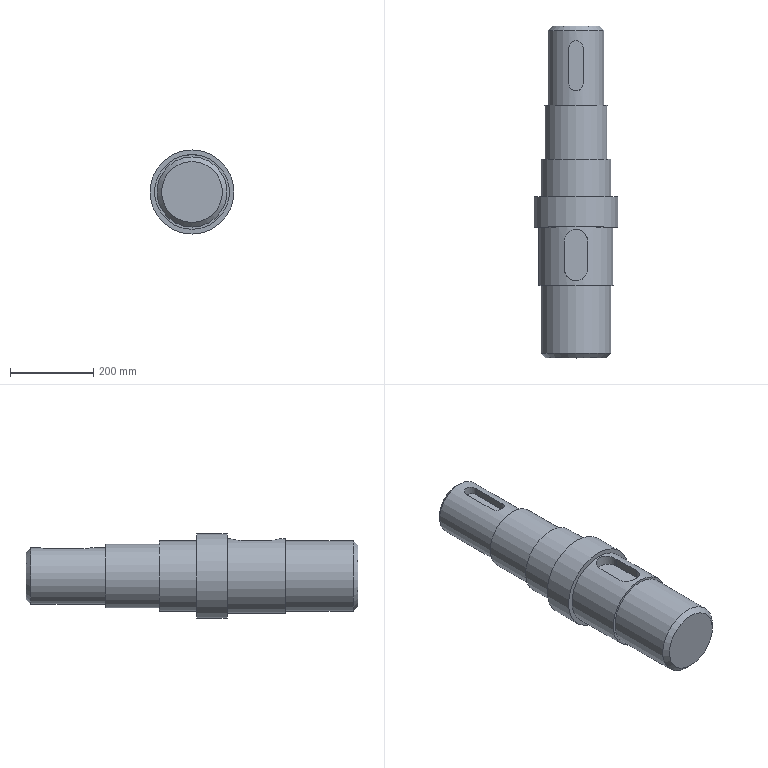Part | NX | features BOSS 5, CHAMFER 2, DATUM_PLANE 2, RECT_SLOT 2, CYLINDER 1, DATUM_CSYS 1, Delete Body 1, LINKED_BODY 1, MOVE_FACE 1, SCALE 1 | 1 solid | 25 faces | box 202.5 x 798.75 x 202.5 mm | volume 16646925 mm3 | plane 13 | cylinder 10 | cone 2 | commonest cylinder face diameters 33.75 x2 56.25 x2 168.75 x2 135 x1 151.875 x1 180 x1
STEP:
#1=CARTESIAN_POINT('',(-1724.979,434.125,-310.332));
#2=VERTEX_POINT('',#1);
#3=CARTESIAN_POINT('',(-1724.979,434.125,-366.582));
#4=DIRECTION('',(0.,1.,0.));
#5=DIRECTION('',(0.,0.,1.));
#6=AXIS2_PLACEMENT_3D('',#3,#4,#5);
#7=CIRCLE('',#6,56.25);
#8=EDGE_CURVE('',#2,#2,#7,.T.);
#9=ORIENTED_EDGE('',*,*,#8,.T.);
#10=EDGE_LOOP('',(#9));
#11=FACE_BOUND('',#10,.T.);
#12=CARTESIAN_POINT('',(-1724.979,434.125,-366.582));
#13=DIRECTION('',(0.,1.,0.));
#14=DIRECTION('',(0.,0.,1.));
#15=AXIS2_PLACEMENT_3D('',#12,#13,#14);
#16=PLANE('',#15);
#17=ADVANCED_FACE('',(#11),#16,.T.);
#18=CARTESIAN_POINT('',(-1741.854,381.851,-301.226));
#19=VERTEX_POINT('',#18);
#20=CARTESIAN_POINT('',(-1741.854,294.976,-301.226));
#21=VERTEX_POINT('',#20);
#22=CARTESIAN_POINT('',(-1741.854,242.875,-301.226));
#23=DIRECTION('',(0.,1.,0.));
#24=VECTOR('',#23,1000.);
#25=LINE('',#22,#24);
#26=EDGE_CURVE('',#19,#21,#25,.F.);
#27=ORIENTED_EDGE('',*,*,#26,.F.);
#28=CARTESIAN_POINT('',(-1708.104,381.851,-301.226));
#29=VERTEX_POINT('',#28);
#30=CARTESIAN_POINT('',(-1708.104,381.851,-301.226));
#31=CARTESIAN_POINT('',(-1708.104,384.09,-301.226));
#32=CARTESIAN_POINT('',(-1708.995,388.496,-300.987));
#33=CARTESIAN_POINT('',(-1712.741,394.093,-300.143));
#34=CARTESIAN_POINT('',(-1718.323,397.833,-299.314));
#35=CARTESIAN_POINT('',(-1724.963,399.17,-298.968));
#36=CARTESIAN_POINT('',(-1731.612,397.845,-299.309));
#37=CARTESIAN_POINT('',(-1739.094,392.847,-300.43));
#38=CARTESIAN_POINT('',(-1741.854,386.329,-301.226));
#39=CARTESIAN_POINT('',(-1741.854,381.851,-301.226));
#40=B_SPLINE_CURVE_WITH_KNOTS('',3,(#30,#31,#32,#33,#34,#35,#36,#37,#38,#39),.UNSPECIFIED.,.F.,.F.,(4,1,1,1,1,1,1,4),(0.,0.006619,0.01324,0.01986,0.02648,0.0331,0.03971,0.05295),.UNSPECIFIED.);
#41=EDGE_CURVE('',#29,#19,#40,.T.);
#42=ORIENTED_EDGE('',*,*,#41,.F.);
#43=CARTESIAN_POINT('',(-1708.104,294.976,-301.226));
#44=VERTEX_POINT('',#43);
#45=CARTESIAN_POINT('',(-1708.104,242.875,-301.226));
#46=DIRECTION('',(0.,1.,0.));
#47=VECTOR('',#46,1000.);
#48=LINE('',#45,#47);
#49=EDGE_CURVE('',#44,#29,#48,.T.);
#50=ORIENTED_EDGE('',*,*,#49,.F.);
#51=CARTESIAN_POINT('',(-1741.854,294.976,-301.226));
#52=CARTESIAN_POINT('',(-1741.854,292.737,-301.226));
#53=CARTESIAN_POINT('',(-1740.964,288.332,-300.987));
#54=CARTESIAN_POINT('',(-1737.218,282.735,-300.143));
#55=CARTESIAN_POINT('',(-1731.636,278.995,-299.314));
#56=CARTESIAN_POINT('',(-1724.996,277.658,-298.968));
#57=CARTESIAN_POINT('',(-1718.347,278.983,-299.309));
#58=CARTESIAN_POINT('',(-1710.865,283.981,-300.43));
#59=CARTESIAN_POINT('',(-1708.104,290.498,-301.226));
#60=CARTESIAN_POINT('',(-1708.104,294.976,-301.226));
#61=B_SPLINE_CURVE_WITH_KNOTS('',3,(#51,#52,#53,#54,#55,#56,#57,#58,#59,#60),.UNSPECIFIED.,.F.,.F.,(4,1,1,1,1,1,1,4),(0.,0.006619,0.01324,0.01986,0.02648,0.0331,0.03971,0.05295),.UNSPECIFIED.);
#62=EDGE_CURVE('',#21,#44,#61,.T.);
#63=ORIENTED_EDGE('',*,*,#62,.F.);
#64=EDGE_LOOP('',(#27,#42,#50,#63));
#65=FACE_BOUND('',#64,.T.);
#66=CARTESIAN_POINT('',(-1724.979,422.875,-299.082));
#67=VERTEX_POINT('',#66);
#68=CARTESIAN_POINT('',(-1724.979,422.875,-366.582));
#69=DIRECTION('',(0.,1.,0.));
#70=DIRECTION('',(0.,0.,1.));
#71=AXIS2_PLACEMENT_3D('',#68,#69,#70);
#72=CIRCLE('',#71,67.5);
#73=EDGE_CURVE('',#67,#67,#72,.F.);
#74=ORIENTED_EDGE('',*,*,#73,.T.);
#75=EDGE_LOOP('',(#74));
#76=FACE_BOUND('',#75,.T.);
#77=CARTESIAN_POINT('',(-1724.979,242.875,-299.082));
#78=VERTEX_POINT('',#77);
#79=CARTESIAN_POINT('',(-1724.979,242.875,-366.582));
#80=DIRECTION('',(0.,1.,0.));
#81=DIRECTION('',(0.,0.,1.));
#82=AXIS2_PLACEMENT_3D('',#79,#80,#81);
#83=CIRCLE('',#82,67.5);
#84=EDGE_CURVE('',#78,#78,#83,.F.);
#85=ORIENTED_EDGE('',*,*,#84,.F.);
#86=EDGE_LOOP('',(#85));
#87=FACE_BOUND('',#86,.T.);
#88=CARTESIAN_POINT('',(-1724.979,242.875,-366.582));
#89=DIRECTION('',(0.,1.,0.));
#90=DIRECTION('',(0.,0.,1.));
#91=AXIS2_PLACEMENT_3D('',#88,#89,#90);
#92=CYLINDRICAL_SURFACE('',#91,67.5);
#93=ADVANCED_FACE('',(#65,#76,#87),#92,.T.);
#94=ORIENTED_EDGE('',*,*,#84,.T.);
#95=EDGE_LOOP('',(#94));
#96=FACE_BOUND('',#95,.T.);
#97=CARTESIAN_POINT('',(-1724.979,242.875,-442.52));
#98=VERTEX_POINT('',#97);
#99=CARTESIAN_POINT('',(-1724.979,242.875,-366.582));
#100=DIRECTION('',(0.,-1.,0.));
#101=DIRECTION('',(0.,0.,-1.));
#102=AXIS2_PLACEMENT_3D('',#99,#100,#101);
#103=CIRCLE('',#102,75.938);
#104=EDGE_CURVE('',#98,#98,#103,.T.);
#105=ORIENTED_EDGE('',*,*,#104,.F.);
#106=EDGE_LOOP('',(#105));
#107=FACE_BOUND('',#106,.T.);
#108=CARTESIAN_POINT('',(-1724.979,242.875,-366.582));
#109=DIRECTION('',(0.,1.,0.));
#110=DIRECTION('',(0.,0.,1.));
#111=AXIS2_PLACEMENT_3D('',#108,#109,#110);
#112=PLANE('',#111);
#113=ADVANCED_FACE('',(#96,#107),#112,.T.);
#114=CARTESIAN_POINT('',(-1724.979,113.5,-442.52));
#115=VERTEX_POINT('',#114);
#116=CARTESIAN_POINT('',(-1724.979,113.5,-366.582));
#117=DIRECTION('',(0.,-1.,0.));
#118=DIRECTION('',(0.,0.,-1.));
#119=AXIS2_PLACEMENT_3D('',#116,#117,#118);
#120=CIRCLE('',#119,75.938);
#121=EDGE_CURVE('',#115,#115,#120,.T.);
#122=ORIENTED_EDGE('',*,*,#121,.F.);
#123=EDGE_LOOP('',(#122));
#124=FACE_BOUND('',#123,.T.);
#125=ORIENTED_EDGE('',*,*,#104,.T.);
#126=EDGE_LOOP('',(#125));
#127=FACE_BOUND('',#126,.T.);
#128=CARTESIAN_POINT('',(-1724.979,242.875,-366.582));
#129=DIRECTION('',(0.,-1.,0.));
#130=DIRECTION('',(0.,0.,-1.));
#131=AXIS2_PLACEMENT_3D('',#128,#129,#130);
#132=CYLINDRICAL_SURFACE('',#131,75.938);
#133=ADVANCED_FACE('',(#124,#127),#132,.T.);
#134=ORIENTED_EDGE('',*,*,#121,.T.);
#135=EDGE_LOOP('',(#134));
#136=FACE_BOUND('',#135,.T.);
#137=CARTESIAN_POINT('',(-1724.979,113.5,-450.957));
#138=VERTEX_POINT('',#137);
#139=CARTESIAN_POINT('',(-1724.979,113.5,-366.582));
#140=DIRECTION('',(0.,-1.,0.));
#141=DIRECTION('',(0.,0.,-1.));
#142=AXIS2_PLACEMENT_3D('',#139,#140,#141);
#143=CIRCLE('',#142,84.375);
#144=EDGE_CURVE('',#138,#138,#143,.T.);
#145=ORIENTED_EDGE('',*,*,#144,.F.);
#146=EDGE_LOOP('',(#145));
#147=FACE_BOUND('',#146,.T.);
#148=CARTESIAN_POINT('',(-1724.979,113.5,-366.582));
#149=DIRECTION('',(0.,1.,0.));
#150=DIRECTION('',(0.,0.,1.));
#151=AXIS2_PLACEMENT_3D('',#148,#149,#150);
#152=PLANE('',#151);
#153=ADVANCED_FACE('',(#136,#147),#152,.T.);
#154=CARTESIAN_POINT('',(-1724.979,23.5,-450.957));
#155=VERTEX_POINT('',#154);
#156=CARTESIAN_POINT('',(-1724.979,23.5,-366.582));
#157=DIRECTION('',(0.,-1.,0.));
#158=DIRECTION('',(0.,0.,-1.));
#159=AXIS2_PLACEMENT_3D('',#156,#157,#158);
#160=CIRCLE('',#159,84.375);
#161=EDGE_CURVE('',#155,#155,#160,.T.);
#162=ORIENTED_EDGE('',*,*,#161,.F.);
#163=EDGE_LOOP('',(#162));
#164=FACE_BOUND('',#163,.T.);
#165=ORIENTED_EDGE('',*,*,#144,.T.);
#166=EDGE_LOOP('',(#165));
#167=FACE_BOUND('',#166,.T.);
#168=CARTESIAN_POINT('',(-1724.979,113.5,-366.582));
#169=DIRECTION('',(0.,-1.,0.));
#170=DIRECTION('',(0.,0.,-1.));
#171=AXIS2_PLACEMENT_3D('',#168,#169,#170);
#172=CYLINDRICAL_SURFACE('',#171,84.375);
#173=ADVANCED_FACE('',(#164,#167),#172,.T.);
#174=CARTESIAN_POINT('',(-1724.979,-49.625,-456.582));
#175=VERTEX_POINT('',#174);
#176=CARTESIAN_POINT('',(-1724.979,-49.625,-366.582));
#177=DIRECTION('',(0.,-1.,0.));
#178=DIRECTION('',(0.,0.,-1.));
#179=AXIS2_PLACEMENT_3D('',#176,#177,#178);
#180=CIRCLE('',#179,90.);
#181=EDGE_CURVE('',#175,#175,#180,.T.);
#182=ORIENTED_EDGE('',*,*,#181,.F.);
#183=EDGE_LOOP('',(#182));
#184=FACE_BOUND('',#183,.T.);
#185=CARTESIAN_POINT('',(-1724.979,-49.625,-467.832));
#186=VERTEX_POINT('',#185);
#187=CARTESIAN_POINT('',(-1724.979,-49.625,-366.582));
#188=DIRECTION('',(0.,-1.,0.));
#189=DIRECTION('',(0.,0.,-1.));
#190=AXIS2_PLACEMENT_3D('',#187,#188,#189);
#191=CIRCLE('',#190,101.25);
#192=EDGE_CURVE('',#186,#186,#191,.T.);
#193=ORIENTED_EDGE('',*,*,#192,.T.);
#194=EDGE_LOOP('',(#193));
#195=FACE_BOUND('',#194,.T.);
#196=CARTESIAN_POINT('',(-1724.979,-49.625,-366.582));
#197=DIRECTION('',(0.,-1.,0.));
#198=DIRECTION('',(0.,0.,-1.));
#199=AXIS2_PLACEMENT_3D('',#196,#197,#198);
#200=PLANE('',#199);
#201=ADVANCED_FACE('',(#184,#195),#200,.T.);
#202=ORIENTED_EDGE('',*,*,#161,.T.);
#203=EDGE_LOOP('',(#202));
#204=FACE_BOUND('',#203,.T.);
#205=CARTESIAN_POINT('',(-1724.979,23.5,-467.832));
#206=VERTEX_POINT('',#205);
#207=CARTESIAN_POINT('',(-1724.979,23.5,-366.582));
#208=DIRECTION('',(0.,-1.,0.));
#209=DIRECTION('',(0.,0.,-1.));
#210=AXIS2_PLACEMENT_3D('',#207,#208,#209);
#211=CIRCLE('',#210,101.25);
#212=EDGE_CURVE('',#206,#206,#211,.T.);
#213=ORIENTED_EDGE('',*,*,#212,.F.);
#214=EDGE_LOOP('',(#213));
#215=FACE_BOUND('',#214,.T.);
#216=CARTESIAN_POINT('',(-1724.979,23.5,-366.582));
#217=DIRECTION('',(0.,1.,0.));
#218=DIRECTION('',(0.,0.,1.));
#219=AXIS2_PLACEMENT_3D('',#216,#217,#218);
#220=PLANE('',#219);
#221=ADVANCED_FACE('',(#204,#215),#220,.T.);
#222=ORIENTED_EDGE('',*,*,#192,.F.);
#223=EDGE_LOOP('',(#222));
#224=FACE_BOUND('',#223,.T.);
#225=ORIENTED_EDGE('',*,*,#212,.T.);
#226=EDGE_LOOP('',(#225));
#227=FACE_BOUND('',#226,.T.);
#228=CARTESIAN_POINT('',(-1724.979,23.5,-366.582));
#229=DIRECTION('',(0.,-1.,0.));
#230=DIRECTION('',(0.,0.,-1.));
#231=AXIS2_PLACEMENT_3D('',#228,#229,#230);
#232=CYLINDRICAL_SURFACE('',#231,101.25);
#233=ADVANCED_FACE('',(#224,#227),#232,.T.);
#234=CARTESIAN_POINT('',(-1724.979,-190.25,-450.957));
#235=VERTEX_POINT('',#234);
#236=CARTESIAN_POINT('',(-1724.979,-190.25,-366.582));
#237=DIRECTION('',(0.,-1.,0.));
#238=DIRECTION('',(0.,0.,-1.));
#239=AXIS2_PLACEMENT_3D('',#236,#237,#238);
#240=CIRCLE('',#239,84.375);
#241=EDGE_CURVE('',#235,#235,#240,.T.);
#242=ORIENTED_EDGE('',*,*,#241,.F.);
#243=EDGE_LOOP('',(#242));
#244=FACE_BOUND('',#243,.T.);
#245=CARTESIAN_POINT('',(-1724.979,-190.25,-456.582));
#246=VERTEX_POINT('',#245);
#247=CARTESIAN_POINT('',(-1724.979,-190.25,-366.582));
#248=DIRECTION('',(0.,-1.,0.));
#249=DIRECTION('',(0.,0.,-1.));
#250=AXIS2_PLACEMENT_3D('',#247,#248,#249);
#251=CIRCLE('',#250,90.);
#252=EDGE_CURVE('',#246,#246,#251,.T.);
#253=ORIENTED_EDGE('',*,*,#252,.T.);
#254=EDGE_LOOP('',(#253));
#255=FACE_BOUND('',#254,.T.);
#256=CARTESIAN_POINT('',(-1724.979,-190.25,-366.582));
#257=DIRECTION('',(0.,-1.,0.));
#258=DIRECTION('',(0.,0.,-1.));
#259=AXIS2_PLACEMENT_3D('',#256,#257,#258);
#260=PLANE('',#259);
#261=ADVANCED_FACE('',(#244,#255),#260,.T.);
#262=CARTESIAN_POINT('',(-1753.104,-83.375,-281.09));
#263=VERTEX_POINT('',#262);
#264=CARTESIAN_POINT('',(-1753.104,-150.875,-281.09));
#265=VERTEX_POINT('',#264);
#266=CARTESIAN_POINT('',(-1753.104,-49.625,-281.09));
#267=DIRECTION('',(0.,-1.,0.));
#268=VECTOR('',#267,1000.);
#269=LINE('',#266,#268);
#270=EDGE_CURVE('',#263,#265,#269,.T.);
#271=ORIENTED_EDGE('',*,*,#270,.F.);
#272=CARTESIAN_POINT('',(-1696.854,-83.375,-281.09));
#273=VERTEX_POINT('',#272);
#274=CARTESIAN_POINT('',(-1696.854,-83.375,-281.09));
#275=CARTESIAN_POINT('',(-1696.854,-81.505,-281.09));
#276=CARTESIAN_POINT('',(-1697.219,-77.839,-280.968));
#277=CARTESIAN_POINT('',(-1699.392,-70.704,-280.278));
#278=CARTESIAN_POINT('',(-1704.582,-62.985,-278.802));
#279=CARTESIAN_POINT('',(-1713.861,-56.747,-277.066));
#280=CARTESIAN_POINT('',(-1724.946,-54.506,-276.342));
#281=CARTESIAN_POINT('',(-1736.061,-56.727,-277.06));
#282=CARTESIAN_POINT('',(-1745.375,-62.976,-278.8));
#283=CARTESIAN_POINT('',(-1751.603,-72.261,-280.575));
#284=CARTESIAN_POINT('',(-1753.104,-79.634,-281.09));
#285=CARTESIAN_POINT('',(-1753.104,-83.375,-281.09));
#286=B_SPLINE_CURVE_WITH_KNOTS('',3,(#274,#275,#276,#277,#278,#279,#280,#281,#282,#283,#284,#285),.UNSPECIFIED.,.F.,.F.,(4,1,1,1,1,1,1,1,1,4),(0.,0.005528,0.01106,0.02211,0.03317,0.04423,0.05528,0.06634,0.0774,0.08846),.UNSPECIFIED.);
#287=EDGE_CURVE('',#273,#263,#286,.T.);
#288=ORIENTED_EDGE('',*,*,#287,.F.);
#289=CARTESIAN_POINT('',(-1696.854,-150.875,-281.09));
#290=VERTEX_POINT('',#289);
#291=CARTESIAN_POINT('',(-1696.854,-49.625,-281.09));
#292=DIRECTION('',(0.,-1.,0.));
#293=VECTOR('',#292,1000.);
#294=LINE('',#291,#293);
#295=EDGE_CURVE('',#290,#273,#294,.F.);
#296=ORIENTED_EDGE('',*,*,#295,.F.);
#297=CARTESIAN_POINT('',(-1753.104,-150.875,-281.09));
#298=CARTESIAN_POINT('',(-1753.104,-152.745,-281.09));
#299=CARTESIAN_POINT('',(-1752.739,-156.411,-280.968));
#300=CARTESIAN_POINT('',(-1750.567,-163.546,-280.278));
#301=CARTESIAN_POINT('',(-1745.377,-171.265,-278.802));
#302=CARTESIAN_POINT('',(-1736.097,-177.503,-277.066));
#303=CARTESIAN_POINT('',(-1725.013,-179.744,-276.342));
#304=CARTESIAN_POINT('',(-1713.897,-177.523,-277.06));
#305=CARTESIAN_POINT('',(-1704.583,-171.274,-278.8));
#306=CARTESIAN_POINT('',(-1698.356,-161.989,-280.575));
#307=CARTESIAN_POINT('',(-1696.854,-154.616,-281.09));
#308=CARTESIAN_POINT('',(-1696.854,-150.875,-281.09));
#309=B_SPLINE_CURVE_WITH_KNOTS('',3,(#297,#298,#299,#300,#301,#302,#303,#304,#305,#306,#307,#308),.UNSPECIFIED.,.F.,.F.,(4,1,1,1,1,1,1,1,1,4),(0.,0.005528,0.01106,0.02211,0.03317,0.04423,0.05528,0.06634,0.0774,0.08846),.UNSPECIFIED.);
#310=EDGE_CURVE('',#265,#290,#309,.T.);
#311=ORIENTED_EDGE('',*,*,#310,.F.);
#312=EDGE_LOOP('',(#271,#288,#296,#311));
#313=FACE_BOUND('',#312,.T.);
#314=ORIENTED_EDGE('',*,*,#252,.F.);
#315=EDGE_LOOP('',(#314));
#316=FACE_BOUND('',#315,.T.);
#317=ORIENTED_EDGE('',*,*,#181,.T.);
#318=EDGE_LOOP('',(#317));
#319=FACE_BOUND('',#318,.T.);
#320=CARTESIAN_POINT('',(-1724.979,-49.625,-366.582));
#321=DIRECTION('',(0.,-1.,0.));
#322=DIRECTION('',(0.,0.,-1.));
#323=AXIS2_PLACEMENT_3D('',#320,#321,#322);
#324=CYLINDRICAL_SURFACE('',#323,90.);
#325=ADVANCED_FACE('',(#313,#316,#319),#324,.T.);
#326=CARTESIAN_POINT('',(-1724.979,-364.625,-439.707));
#327=VERTEX_POINT('',#326);
#328=CARTESIAN_POINT('',(-1724.979,-364.625,-366.582));
#329=DIRECTION('',(0.,-1.,0.));
#330=DIRECTION('',(0.,0.,-1.));
#331=AXIS2_PLACEMENT_3D('',#328,#329,#330);
#332=CIRCLE('',#331,73.125);
#333=EDGE_CURVE('',#327,#327,#332,.T.);
#334=ORIENTED_EDGE('',*,*,#333,.T.);
#335=EDGE_LOOP('',(#334));
#336=FACE_BOUND('',#335,.T.);
#337=CARTESIAN_POINT('',(-1724.979,-364.625,-366.582));
#338=DIRECTION('',(0.,-1.,0.));
#339=DIRECTION('',(0.,0.,-1.));
#340=AXIS2_PLACEMENT_3D('',#337,#338,#339);
#341=PLANE('',#340);
#342=ADVANCED_FACE('',(#336),#341,.T.);
#343=CARTESIAN_POINT('',(-1724.979,-353.375,-450.957));
#344=VERTEX_POINT('',#343);
#345=CARTESIAN_POINT('',(-1724.979,-353.375,-366.582));
#346=DIRECTION('',(0.,-1.,0.));
#347=DIRECTION('',(0.,0.,-1.));
#348=AXIS2_PLACEMENT_3D('',#345,#346,#347);
#349=CIRCLE('',#348,84.375);
#350=EDGE_CURVE('',#344,#344,#349,.F.);
#351=ORIENTED_EDGE('',*,*,#350,.T.);
#352=EDGE_LOOP('',(#351));
#353=FACE_BOUND('',#352,.T.);
#354=ORIENTED_EDGE('',*,*,#241,.T.);
#355=EDGE_LOOP('',(#354));
#356=FACE_BOUND('',#355,.T.);
#357=CARTESIAN_POINT('',(-1724.979,-190.25,-366.582));
#358=DIRECTION('',(0.,-1.,0.));
#359=DIRECTION('',(0.,0.,-1.));
#360=AXIS2_PLACEMENT_3D('',#357,#358,#359);
#361=CYLINDRICAL_SURFACE('',#360,84.375);
#362=ADVANCED_FACE('',(#353,#356),#361,.T.);
#363=ORIENTED_EDGE('',*,*,#350,.F.);
#364=EDGE_LOOP('',(#363));
#365=FACE_BOUND('',#364,.T.);
#366=ORIENTED_EDGE('',*,*,#333,.F.);
#367=EDGE_LOOP('',(#366));
#368=FACE_BOUND('',#367,.T.);
#369=CARTESIAN_POINT('',(-1724.979,-364.625,-366.582));
#370=DIRECTION('',(0.,1.,0.));
#371=DIRECTION('',(0.,0.,1.));
#372=AXIS2_PLACEMENT_3D('',#369,#370,#371);
#373=CONICAL_SURFACE('',#372,73.125,0.7854);
#374=ADVANCED_FACE('',(#365,#368),#373,.T.);
#375=ORIENTED_EDGE('',*,*,#8,.F.);
#376=EDGE_LOOP('',(#375));
#377=FACE_BOUND('',#376,.T.);
#378=ORIENTED_EDGE('',*,*,#73,.F.);
#379=EDGE_LOOP('',(#378));
#380=FACE_BOUND('',#379,.T.);
#381=CARTESIAN_POINT('',(-1724.979,422.875,-366.582));
#382=DIRECTION('',(0.,-1.,0.));
#383=DIRECTION('',(0.,0.,-1.));
#384=AXIS2_PLACEMENT_3D('',#381,#382,#383);
#385=CONICAL_SURFACE('',#384,67.5,0.7854);
#386=ADVANCED_FACE('',(#377,#380),#385,.T.);
#387=ORIENTED_EDGE('',*,*,#26,.T.);
#388=CARTESIAN_POINT('',(-1741.854,294.976,-318.77));
#389=VERTEX_POINT('',#388);
#390=CARTESIAN_POINT('',(-1741.854,294.976,-299.082));
#391=DIRECTION('',(0.,0.,1.));
#392=VECTOR('',#391,1000.);
#393=LINE('',#390,#392);
#394=EDGE_CURVE('',#21,#389,#393,.F.);
#395=ORIENTED_EDGE('',*,*,#394,.T.);
#396=CARTESIAN_POINT('',(-1741.854,381.851,-318.77));
#397=VERTEX_POINT('',#396);
#398=CARTESIAN_POINT('',(-1741.854,274.976,-318.77));
#399=DIRECTION('',(0.,1.,0.));
#400=VECTOR('',#399,1000.);
#401=LINE('',#398,#400);
#402=EDGE_CURVE('',#397,#389,#401,.F.);
#403=ORIENTED_EDGE('',*,*,#402,.F.);
#404=CARTESIAN_POINT('',(-1741.854,381.851,-299.082));
#405=DIRECTION('',(0.,0.,1.));
#406=VECTOR('',#405,1000.);
#407=LINE('',#404,#406);
#408=EDGE_CURVE('',#19,#397,#407,.F.);
#409=ORIENTED_EDGE('',*,*,#408,.F.);
#410=EDGE_LOOP('',(#387,#395,#403,#409));
#411=FACE_BOUND('',#410,.T.);
#412=CARTESIAN_POINT('',(-1741.854,328.414,-299.082));
#413=DIRECTION('',(-1.,0.,0.));
#414=DIRECTION('',(0.,0.,1.));
#415=AXIS2_PLACEMENT_3D('',#412,#413,#414);
#416=PLANE('',#415);
#417=ADVANCED_FACE('',(#411),#416,.F.);
#418=ORIENTED_EDGE('',*,*,#402,.T.);
#419=CARTESIAN_POINT('',(-1708.104,294.976,-318.77));
#420=VERTEX_POINT('',#419);
#421=CARTESIAN_POINT('',(-1724.979,294.976,-318.77));
#422=DIRECTION('',(0.,0.,1.));
#423=DIRECTION('',(1.,0.,0.));
#424=AXIS2_PLACEMENT_3D('',#421,#422,#423);
#425=CIRCLE('',#424,16.875);
#426=EDGE_CURVE('',#420,#389,#425,.F.);
#427=ORIENTED_EDGE('',*,*,#426,.F.);
#428=CARTESIAN_POINT('',(-1708.104,381.851,-318.77));
#429=VERTEX_POINT('',#428);
#430=CARTESIAN_POINT('',(-1708.104,274.976,-318.77));
#431=DIRECTION('',(0.,1.,0.));
#432=VECTOR('',#431,1000.);
#433=LINE('',#430,#432);
#434=EDGE_CURVE('',#429,#420,#433,.F.);
#435=ORIENTED_EDGE('',*,*,#434,.F.);
#436=CARTESIAN_POINT('',(-1724.979,381.851,-318.77));
#437=DIRECTION('',(0.,0.,1.));
#438=DIRECTION('',(1.,0.,0.));
#439=AXIS2_PLACEMENT_3D('',#436,#437,#438);
#440=CIRCLE('',#439,16.875);
#441=EDGE_CURVE('',#397,#429,#440,.F.);
#442=ORIENTED_EDGE('',*,*,#441,.F.);
#443=EDGE_LOOP('',(#418,#427,#435,#442));
#444=FACE_BOUND('',#443,.T.);
#445=CARTESIAN_POINT('',(-1724.979,328.414,-318.77));
#446=DIRECTION('',(0.,0.,-1.));
#447=DIRECTION('',(-1.,0.,0.));
#448=AXIS2_PLACEMENT_3D('',#445,#446,#447);
#449=PLANE('',#448);
#450=ADVANCED_FACE('',(#444),#449,.F.);
#451=ORIENTED_EDGE('',*,*,#394,.F.);
#452=ORIENTED_EDGE('',*,*,#62,.T.);
#453=CARTESIAN_POINT('',(-1708.104,294.976,-299.082));
#454=DIRECTION('',(0.,0.,1.));
#455=VECTOR('',#454,1000.);
#456=LINE('',#453,#455);
#457=EDGE_CURVE('',#44,#420,#456,.F.);
#458=ORIENTED_EDGE('',*,*,#457,.T.);
#459=ORIENTED_EDGE('',*,*,#426,.T.);
#460=EDGE_LOOP('',(#451,#452,#458,#459));
#461=FACE_BOUND('',#460,.T.);
#462=CARTESIAN_POINT('',(-1724.979,294.976,-299.082));
#463=DIRECTION('',(0.,0.,1.));
#464=DIRECTION('',(1.,0.,0.));
#465=AXIS2_PLACEMENT_3D('',#462,#463,#464);
#466=CYLINDRICAL_SURFACE('',#465,16.875);
#467=ADVANCED_FACE('',(#461),#466,.F.);
#468=ORIENTED_EDGE('',*,*,#49,.T.);
#469=CARTESIAN_POINT('',(-1708.104,381.851,-299.082));
#470=DIRECTION('',(0.,0.,1.));
#471=VECTOR('',#470,1000.);
#472=LINE('',#469,#471);
#473=EDGE_CURVE('',#29,#429,#472,.F.);
#474=ORIENTED_EDGE('',*,*,#473,.T.);
#475=ORIENTED_EDGE('',*,*,#434,.T.);
#476=ORIENTED_EDGE('',*,*,#457,.F.);
#477=EDGE_LOOP('',(#468,#474,#475,#476));
#478=FACE_BOUND('',#477,.T.);
#479=CARTESIAN_POINT('',(-1708.104,328.414,-299.082));
#480=DIRECTION('',(1.,0.,0.));
#481=DIRECTION('',(0.,0.,-1.));
#482=AXIS2_PLACEMENT_3D('',#479,#480,#481);
#483=PLANE('',#482);
#484=ADVANCED_FACE('',(#478),#483,.F.);
#485=ORIENTED_EDGE('',*,*,#473,.F.);
#486=ORIENTED_EDGE('',*,*,#41,.T.);
#487=ORIENTED_EDGE('',*,*,#408,.T.);
#488=ORIENTED_EDGE('',*,*,#441,.T.);
#489=EDGE_LOOP('',(#485,#486,#487,#488));
#490=FACE_BOUND('',#489,.T.);
#491=CARTESIAN_POINT('',(-1724.979,381.851,-299.082));
#492=DIRECTION('',(0.,0.,1.));
#493=DIRECTION('',(1.,0.,0.));
#494=AXIS2_PLACEMENT_3D('',#491,#492,#493);
#495=CYLINDRICAL_SURFACE('',#494,16.875);
#496=ADVANCED_FACE('',(#490),#495,.F.);
#497=ORIENTED_EDGE('',*,*,#270,.T.);
#498=CARTESIAN_POINT('',(-1753.104,-150.875,-301.895));
#499=VERTEX_POINT('',#498);
#500=CARTESIAN_POINT('',(-1753.104,-150.875,-276.582));
#501=DIRECTION('',(0.,0.,1.));
#502=VECTOR('',#501,1000.);
#503=LINE('',#500,#502);
#504=EDGE_CURVE('',#265,#499,#503,.F.);
#505=ORIENTED_EDGE('',*,*,#504,.T.);
#506=CARTESIAN_POINT('',(-1753.104,-83.375,-301.895));
#507=VERTEX_POINT('',#506);
#508=CARTESIAN_POINT('',(-1753.104,-150.875,-301.895));
#509=DIRECTION('',(0.,1.,0.));
#510=VECTOR('',#509,1000.);
#511=LINE('',#508,#510);
#512=EDGE_CURVE('',#507,#499,#511,.F.);
#513=ORIENTED_EDGE('',*,*,#512,.F.);
#514=CARTESIAN_POINT('',(-1753.104,-83.375,-276.582));
#515=DIRECTION('',(0.,0.,1.));
#516=VECTOR('',#515,1000.);
#517=LINE('',#514,#516);
#518=EDGE_CURVE('',#263,#507,#517,.F.);
#519=ORIENTED_EDGE('',*,*,#518,.F.);
#520=EDGE_LOOP('',(#497,#505,#513,#519));
#521=FACE_BOUND('',#520,.T.);
#522=CARTESIAN_POINT('',(-1753.104,-117.125,-276.582));
#523=DIRECTION('',(-1.,0.,0.));
#524=DIRECTION('',(0.,0.,1.));
#525=AXIS2_PLACEMENT_3D('',#522,#523,#524);
#526=PLANE('',#525);
#527=ADVANCED_FACE('',(#521),#526,.F.);
#528=ORIENTED_EDGE('',*,*,#512,.T.);
#529=CARTESIAN_POINT('',(-1696.854,-150.875,-301.895));
#530=VERTEX_POINT('',#529);
#531=CARTESIAN_POINT('',(-1724.979,-150.875,-301.895));
#532=DIRECTION('',(0.,0.,1.));
#533=DIRECTION('',(1.,0.,0.));
#534=AXIS2_PLACEMENT_3D('',#531,#532,#533);
#535=CIRCLE('',#534,28.125);
#536=EDGE_CURVE('',#530,#499,#535,.F.);
#537=ORIENTED_EDGE('',*,*,#536,.F.);
#538=CARTESIAN_POINT('',(-1696.854,-83.375,-301.895));
#539=VERTEX_POINT('',#538);
#540=CARTESIAN_POINT('',(-1696.854,-150.875,-301.895));
#541=DIRECTION('',(0.,1.,0.));
#542=VECTOR('',#541,1000.);
#543=LINE('',#540,#542);
#544=EDGE_CURVE('',#539,#530,#543,.F.);
#545=ORIENTED_EDGE('',*,*,#544,.F.);
#546=CARTESIAN_POINT('',(-1724.979,-83.375,-301.895));
#547=DIRECTION('',(0.,0.,1.));
#548=DIRECTION('',(1.,0.,0.));
#549=AXIS2_PLACEMENT_3D('',#546,#547,#548);
#550=CIRCLE('',#549,28.125);
#551=EDGE_CURVE('',#507,#539,#550,.F.);
#552=ORIENTED_EDGE('',*,*,#551,.F.);
#553=EDGE_LOOP('',(#528,#537,#545,#552));
#554=FACE_BOUND('',#553,.T.);
#555=CARTESIAN_POINT('',(-1724.979,-117.125,-301.895));
#556=DIRECTION('',(0.,0.,-1.));
#557=DIRECTION('',(-1.,0.,0.));
#558=AXIS2_PLACEMENT_3D('',#555,#556,#557);
#559=PLANE('',#558);
#560=ADVANCED_FACE('',(#554),#559,.F.);
#561=ORIENTED_EDGE('',*,*,#504,.F.);
#562=ORIENTED_EDGE('',*,*,#310,.T.);
#563=CARTESIAN_POINT('',(-1696.854,-150.875,-276.582));
#564=DIRECTION('',(0.,0.,1.));
#565=VECTOR('',#564,1000.);
#566=LINE('',#563,#565);
#567=EDGE_CURVE('',#290,#530,#566,.F.);
#568=ORIENTED_EDGE('',*,*,#567,.T.);
#569=ORIENTED_EDGE('',*,*,#536,.T.);
#570=EDGE_LOOP('',(#561,#562,#568,#569));
#571=FACE_BOUND('',#570,.T.);
#572=CARTESIAN_POINT('',(-1724.979,-150.875,-276.582));
#573=DIRECTION('',(0.,0.,1.));
#574=DIRECTION('',(1.,0.,0.));
#575=AXIS2_PLACEMENT_3D('',#572,#573,#574);
#576=CYLINDRICAL_SURFACE('',#575,28.125);
#577=ADVANCED_FACE('',(#571),#576,.F.);
#578=ORIENTED_EDGE('',*,*,#295,.T.);
#579=CARTESIAN_POINT('',(-1696.854,-83.375,-276.582));
#580=DIRECTION('',(0.,0.,1.));
#581=VECTOR('',#580,1000.);
#582=LINE('',#579,#581);
#583=EDGE_CURVE('',#273,#539,#582,.F.);
#584=ORIENTED_EDGE('',*,*,#583,.T.);
#585=ORIENTED_EDGE('',*,*,#544,.T.);
#586=ORIENTED_EDGE('',*,*,#567,.F.);
#587=EDGE_LOOP('',(#578,#584,#585,#586));
#588=FACE_BOUND('',#587,.T.);
#589=CARTESIAN_POINT('',(-1696.854,-117.125,-276.582));
#590=DIRECTION('',(1.,0.,0.));
#591=DIRECTION('',(0.,0.,-1.));
#592=AXIS2_PLACEMENT_3D('',#589,#590,#591);
#593=PLANE('',#592);
#594=ADVANCED_FACE('',(#588),#593,.F.);
#595=ORIENTED_EDGE('',*,*,#583,.F.);
#596=ORIENTED_EDGE('',*,*,#287,.T.);
#597=ORIENTED_EDGE('',*,*,#518,.T.);
#598=ORIENTED_EDGE('',*,*,#551,.T.);
#599=EDGE_LOOP('',(#595,#596,#597,#598));
#600=FACE_BOUND('',#599,.T.);
#601=CARTESIAN_POINT('',(-1724.979,-83.375,-276.582));
#602=DIRECTION('',(0.,0.,1.));
#603=DIRECTION('',(1.,0.,0.));
#604=AXIS2_PLACEMENT_3D('',#601,#602,#603);
#605=CYLINDRICAL_SURFACE('',#604,28.125);
#606=ADVANCED_FACE('',(#600),#605,.F.);
#607=CLOSED_SHELL('',(#17,#93,#113,#133,#153,#173,#201,#221,#233,#261,#325,#342,#362,#374,#386,#417,#450,#467,#484,#496,#527,#560,#577,#594,#606));
#608=MANIFOLD_SOLID_BREP('',#607);
#609=(LENGTH_UNIT()NAMED_UNIT(*)SI_UNIT(.MILLI.,.METRE.));
#610=UNCERTAINTY_MEASURE_WITH_UNIT(LENGTH_MEASURE(0.0508),#609,'','');
#611=(NAMED_UNIT(*)PLANE_ANGLE_UNIT()SI_UNIT($,.RADIAN.));
#612=(NAMED_UNIT(*)SI_UNIT($,.STERADIAN.)SOLID_ANGLE_UNIT());
#613=(GEOMETRIC_REPRESENTATION_CONTEXT(3)GLOBAL_UNCERTAINTY_ASSIGNED_CONTEXT((#610))GLOBAL_UNIT_ASSIGNED_CONTEXT((#609,#611,#612))REPRESENTATION_CONTEXT('',''));
#614=ADVANCED_BREP_SHAPE_REPRESENTATION('',(#608),#613);